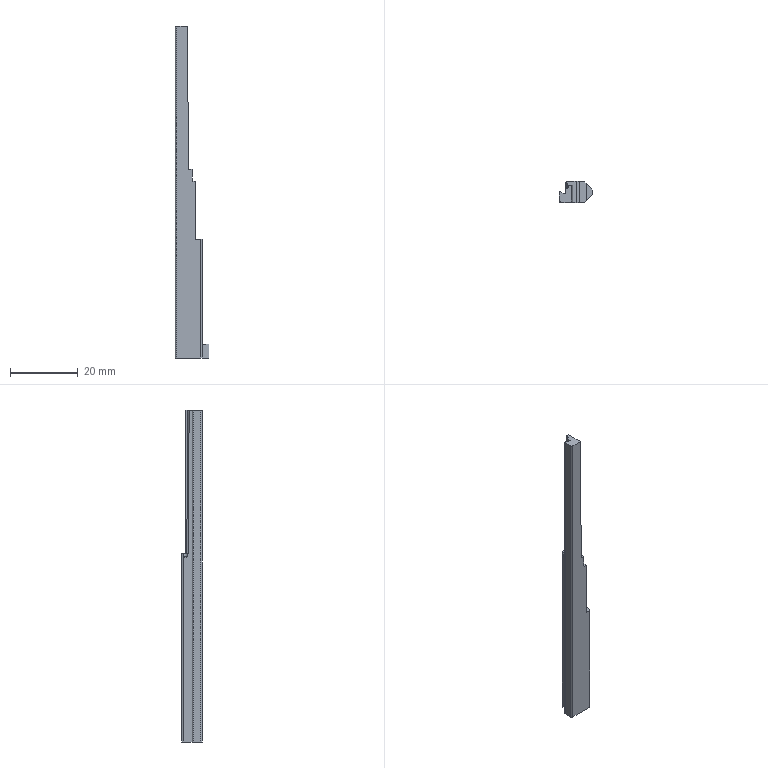Part | Creo | 1 solid | 32 faces | box 10 x 6.2 x 98.191 mm | volume 2714 mm3 | plane 25 | cylinder 5 | cone 2 | commonest cylinder face diameters 0.6 x2 1 x2 1.005 x1
STEP:
#1=CARTESIAN_POINT('',(0.,0.,0.));
#2=DIRECTION('',(0.,0.,1.));
#3=DIRECTION('',(1.,0.,0.));
#4=AXIS2_PLACEMENT_3D('',#1,#2,#3);
#5=CARTESIAN_POINT('',(41.857,15.007,44.101));
#6=VERTEX_POINT('',#5);
#7=CARTESIAN_POINT('',(41.709,15.153,1.79));
#8=VERTEX_POINT('',#7);
#9=CARTESIAN_POINT('',(41.857,15.007,44.101));
#10=DIRECTION('',(-0.003491,0.00346,-1.));
#11=VECTOR('',#10,42.311);
#12=LINE('',#9,#11);
#13=EDGE_CURVE('',#6,#8,#12,.T.);
#14=ORIENTED_EDGE('',*,*,#13,.T.);
#15=CARTESIAN_POINT('',(43.119,15.166,1.79));
#16=VERTEX_POINT('',#15);
#17=CARTESIAN_POINT('',(43.119,15.166,1.79));
#18=DIRECTION('',(-1.,-0.008727,0.));
#19=VECTOR('',#18,1.41);
#20=LINE('',#17,#19);
#21=EDGE_CURVE('',#16,#8,#20,.T.);
#22=ORIENTED_EDGE('',*,*,#21,.F.);
#23=CARTESIAN_POINT('',(42.75,15.015,44.101));
#24=VERTEX_POINT('',#23);
#25=CARTESIAN_POINT('',(42.75,15.015,44.101));
#26=DIRECTION('',(0.008726,0.003567,-1.));
#27=VECTOR('',#26,42.312);
#28=LINE('',#25,#27);
#29=EDGE_CURVE('',#24,#16,#28,.T.);
#30=ORIENTED_EDGE('',*,*,#29,.F.);
#31=CARTESIAN_POINT('',(42.75,15.015,44.101));
#32=DIRECTION('',(-1.,-0.008727,0.));
#33=VECTOR('',#32,0.8934);
#34=LINE('',#31,#33);
#35=EDGE_CURVE('',#24,#6,#34,.T.);
#36=ORIENTED_EDGE('',*,*,#35,.T.);
#37=EDGE_LOOP('',(#14,#22,#30,#36));
#38=FACE_OUTER_BOUND('',#37,.F.);
#39=CARTESIAN_POINT('',(45.746,15.067,36.563));
#40=DIRECTION('',(0.008726,-1.,-0.003491));
#41=DIRECTION('',(1.,0.008727,0.));
#42=AXIS2_PLACEMENT_3D('',#39,#40,#41);
#43=PLANE('',#42);
#44=ADVANCED_FACE('',(#38),#43,.F.);
#45=CARTESIAN_POINT('',(41.709,14.663,1.79));
#46=VERTEX_POINT('',#45);
#47=CARTESIAN_POINT('',(41.857,14.516,44.101));
#48=VERTEX_POINT('',#47);
#49=CARTESIAN_POINT('',(41.709,14.663,1.79));
#50=DIRECTION('',(0.003491,-0.003491,1.));
#51=VECTOR('',#50,42.311);
#52=LINE('',#49,#51);
#53=EDGE_CURVE('',#46,#48,#52,.T.);
#54=ORIENTED_EDGE('',*,*,#53,.F.);
#55=CARTESIAN_POINT('',(41.709,15.153,1.79));
#56=DIRECTION('',(0.,-1.,-0.000000002));
#57=VECTOR('',#56,0.49);
#58=LINE('',#55,#57);
#59=EDGE_CURVE('',#8,#46,#58,.T.);
#60=ORIENTED_EDGE('',*,*,#59,.F.);
#61=ORIENTED_EDGE('',*,*,#13,.F.);
#62=CARTESIAN_POINT('',(41.857,15.007,44.101));
#63=DIRECTION('',(0.,-1.,-0.000000002));
#64=VECTOR('',#63,0.4913);
#65=LINE('',#62,#64);
#66=EDGE_CURVE('',#6,#48,#65,.T.);
#67=ORIENTED_EDGE('',*,*,#66,.T.);
#68=EDGE_LOOP('',(#54,#60,#61,#67));
#69=FACE_OUTER_BOUND('',#68,.F.);
#70=CARTESIAN_POINT('',(41.83,17.654,36.563));
#71=DIRECTION('',(1.,0.,-0.003491));
#72=DIRECTION('',(0.,1.,0.));
#73=AXIS2_PLACEMENT_3D('',#70,#71,#72);
#74=PLANE('',#73);
#75=ADVANCED_FACE('',(#69),#74,.F.);
#76=CARTESIAN_POINT('',(41.354,14.013,44.101));
#77=VERTEX_POINT('',#76);
#78=CARTESIAN_POINT('',(41.206,14.161,1.79));
#79=VERTEX_POINT('',#78);
#80=CARTESIAN_POINT('',(41.354,14.013,44.101));
#81=DIRECTION('',(-0.003491,0.003491,-1.));
#82=VECTOR('',#81,42.311);
#83=LINE('',#80,#82);
#84=EDGE_CURVE('',#77,#79,#83,.T.);
#85=ORIENTED_EDGE('',*,*,#84,.T.);
#86=CARTESIAN_POINT('',(41.709,14.663,1.79));
#87=CARTESIAN_POINT('',(41.709,14.496,1.79));
#88=CARTESIAN_POINT('',(41.582,14.288,1.79));
#89=CARTESIAN_POINT('',(41.374,14.161,1.79));
#90=CARTESIAN_POINT('',(41.206,14.161,1.79));
#91=B_SPLINE_CURVE_WITH_KNOTS('',3,(#86,#87,#88,#89,#90),.UNSPECIFIED.,.F.,.F.,(4,1,4),(0.,0.5,1.),.UNSPECIFIED.);
#92=EDGE_CURVE('',#46,#79,#91,.T.);
#93=ORIENTED_EDGE('',*,*,#92,.F.);
#94=ORIENTED_EDGE('',*,*,#53,.T.);
#95=CARTESIAN_POINT('',(41.354,14.013,44.101));
#96=CARTESIAN_POINT('',(41.522,14.013,44.101));
#97=CARTESIAN_POINT('',(41.73,14.14,44.101));
#98=CARTESIAN_POINT('',(41.857,14.348,44.101));
#99=CARTESIAN_POINT('',(41.857,14.516,44.101));
#100=B_SPLINE_CURVE_WITH_KNOTS('',3,(#95,#96,#97,#98,#99),.UNSPECIFIED.,.F.,.F.,(4,1,4),(0.,0.5,1.),.UNSPECIFIED.);
#101=EDGE_CURVE('',#77,#48,#100,.T.);
#102=ORIENTED_EDGE('',*,*,#101,.F.);
#103=EDGE_LOOP('',(#85,#93,#94,#102));
#104=FACE_OUTER_BOUND('',#103,.F.);
#105=CARTESIAN_POINT('',(40.869,15.001,-94.88));
#106=DIRECTION('',(0.003491,-0.003491,1.));
#107=DIRECTION('',(0.,1.,0.003491));
#108=AXIS2_PLACEMENT_3D('',#105,#106,#107);
#109=CYLINDRICAL_SURFACE('',#108,0.5025);
#110=ADVANCED_FACE('',(#104),#109,.F.);
#111=CARTESIAN_POINT('',(41.127,14.161,1.79));
#112=VERTEX_POINT('',#111);
#113=CARTESIAN_POINT('',(41.206,14.161,1.79));
#114=DIRECTION('',(-1.,0.,0.));
#115=VECTOR('',#114,0.07962);
#116=LINE('',#113,#115);
#117=EDGE_CURVE('',#79,#112,#116,.T.);
#118=ORIENTED_EDGE('',*,*,#117,.F.);
#119=ORIENTED_EDGE('',*,*,#84,.F.);
#120=CARTESIAN_POINT('',(41.127,14.013,44.101));
#121=VERTEX_POINT('',#120);
#122=CARTESIAN_POINT('',(41.354,14.013,44.101));
#123=DIRECTION('',(-1.,0.,0.000000003));
#124=VECTOR('',#123,0.2273);
#125=LINE('',#122,#124);
#126=EDGE_CURVE('',#77,#121,#125,.T.);
#127=ORIENTED_EDGE('',*,*,#126,.T.);
#128=CARTESIAN_POINT('',(41.127,14.013,44.101));
#129=DIRECTION('',(0.,0.003491,-1.));
#130=VECTOR('',#129,42.311);
#131=LINE('',#128,#130);
#132=EDGE_CURVE('',#121,#112,#131,.T.);
#133=ORIENTED_EDGE('',*,*,#132,.T.);
#134=EDGE_LOOP('',(#118,#119,#127,#133));
#135=FACE_OUTER_BOUND('',#134,.F.);
#136=CARTESIAN_POINT('',(44.44,14.039,36.563));
#137=DIRECTION('',(0.,-1.,-0.003491));
#138=DIRECTION('',(1.,0.,0.));
#139=AXIS2_PLACEMENT_3D('',#136,#137,#138);
#140=PLANE('',#139);
#141=ADVANCED_FACE('',(#135),#140,.F.);
#142=CARTESIAN_POINT('',(43.119,10.049,1.79));
#143=VERTEX_POINT('',#142);
#144=CARTESIAN_POINT('',(44.165,10.049,1.79));
#145=VERTEX_POINT('',#144);
#146=CARTESIAN_POINT('',(43.119,10.049,1.79));
#147=DIRECTION('',(1.,0.,0.));
#148=VECTOR('',#147,1.045);
#149=LINE('',#146,#148);
#150=EDGE_CURVE('',#143,#145,#149,.T.);
#151=ORIENTED_EDGE('',*,*,#150,.F.);
#152=CARTESIAN_POINT('',(43.119,10.049,1.79));
#153=DIRECTION('',(0.,1.,0.));
#154=VECTOR('',#153,5.117);
#155=LINE('',#152,#154);
#156=EDGE_CURVE('',#143,#16,#155,.T.);
#157=ORIENTED_EDGE('',*,*,#156,.T.);
#158=ORIENTED_EDGE('',*,*,#21,.T.);
#159=ORIENTED_EDGE('',*,*,#59,.T.);
#160=ORIENTED_EDGE('',*,*,#92,.T.);
#161=ORIENTED_EDGE('',*,*,#117,.T.);
#162=CARTESIAN_POINT('',(41.127,14.552,1.79));
#163=VERTEX_POINT('',#162);
#164=CARTESIAN_POINT('',(41.127,14.161,1.79));
#165=DIRECTION('',(0.,1.,0.));
#166=VECTOR('',#165,0.3912);
#167=LINE('',#164,#166);
#168=EDGE_CURVE('',#112,#163,#167,.T.);
#169=ORIENTED_EDGE('',*,*,#168,.T.);
#170=CARTESIAN_POINT('',(41.127,15.657,1.79));
#171=VERTEX_POINT('',#170);
#172=CARTESIAN_POINT('',(41.127,15.105,1.79));
#173=DIRECTION('',(0.,0.,-1.));
#174=DIRECTION('',(0.,1.,0.));
#175=AXIS2_PLACEMENT_3D('',#172,#173,#174);
#176=CIRCLE('',#175,0.5527);
#177=EDGE_CURVE('',#171,#163,#176,.T.);
#178=ORIENTED_EDGE('',*,*,#177,.F.);
#179=CARTESIAN_POINT('',(41.127,15.749,1.79));
#180=VERTEX_POINT('',#179);
#181=CARTESIAN_POINT('',(41.127,15.657,1.79));
#182=DIRECTION('',(0.,1.,0.));
#183=VECTOR('',#182,0.09123);
#184=LINE('',#181,#183);
#185=EDGE_CURVE('',#171,#180,#184,.T.);
#186=ORIENTED_EDGE('',*,*,#185,.T.);
#187=CARTESIAN_POINT('',(41.627,16.249,1.79));
#188=VERTEX_POINT('',#187);
#189=CARTESIAN_POINT('',(41.627,15.749,1.79));
#190=DIRECTION('',(0.,0.,1.));
#191=DIRECTION('',(0.,1.,0.));
#192=AXIS2_PLACEMENT_3D('',#189,#190,#191);
#193=CIRCLE('',#192,0.5);
#194=EDGE_CURVE('',#188,#180,#193,.T.);
#195=ORIENTED_EDGE('',*,*,#194,.F.);
#196=CARTESIAN_POINT('',(44.165,16.249,1.79));
#197=VERTEX_POINT('',#196);
#198=CARTESIAN_POINT('',(41.627,16.249,1.79));
#199=DIRECTION('',(1.,0.,0.));
#200=VECTOR('',#199,2.538);
#201=LINE('',#198,#200);
#202=EDGE_CURVE('',#188,#197,#201,.T.);
#203=ORIENTED_EDGE('',*,*,#202,.T.);
#204=CARTESIAN_POINT('',(44.165,16.249,1.79));
#205=DIRECTION('',(0.,-1.,0.));
#206=VECTOR('',#205,6.2);
#207=LINE('',#204,#206);
#208=EDGE_CURVE('',#197,#145,#207,.T.);
#209=ORIENTED_EDGE('',*,*,#208,.T.);
#210=EDGE_LOOP('',(#151,#157,#158,#159,#160,#161,#169,#178,#186,#195,#203,#209));
#211=FACE_OUTER_BOUND('',#210,.F.);
#212=CARTESIAN_POINT('',(-0.07825,87.525,1.79));
#213=DIRECTION('',(0.,0.,-1.));
#214=DIRECTION('',(0.,-1.,0.));
#215=AXIS2_PLACEMENT_3D('',#212,#213,#214);
#216=PLANE('',#215);
#217=ADVANCED_FACE('',(#211),#216,.F.);
#218=CARTESIAN_POINT('',(39.627,10.049,-54.09));
#219=VERTEX_POINT('',#218);
#220=CARTESIAN_POINT('',(46.627,10.049,-54.09));
#221=VERTEX_POINT('',#220);
#222=CARTESIAN_POINT('',(39.627,10.049,-54.09));
#223=DIRECTION('',(1.,0.,0.));
#224=VECTOR('',#223,7.);
#225=LINE('',#222,#224);
#226=EDGE_CURVE('',#219,#221,#225,.T.);
#227=ORIENTED_EDGE('',*,*,#226,.F.);
#228=CARTESIAN_POINT('',(39.627,10.049,44.101));
#229=VERTEX_POINT('',#228);
#230=CARTESIAN_POINT('',(39.627,10.049,-54.09));
#231=DIRECTION('',(0.,0.,1.));
#232=VECTOR('',#231,98.191);
#233=LINE('',#230,#232);
#234=EDGE_CURVE('',#219,#229,#233,.T.);
#235=ORIENTED_EDGE('',*,*,#234,.T.);
#236=CARTESIAN_POINT('',(42.75,10.049,44.101));
#237=VERTEX_POINT('',#236);
#238=CARTESIAN_POINT('',(42.75,10.049,44.101));
#239=DIRECTION('',(-1.,0.,0.));
#240=VECTOR('',#239,3.123);
#241=LINE('',#238,#240);
#242=EDGE_CURVE('',#237,#229,#241,.T.);
#243=ORIENTED_EDGE('',*,*,#242,.F.);
#244=CARTESIAN_POINT('',(43.119,10.049,1.79));
#245=DIRECTION('',(-0.008727,0.,1.));
#246=VECTOR('',#245,42.312);
#247=LINE('',#244,#246);
#248=EDGE_CURVE('',#143,#237,#247,.T.);
#249=ORIENTED_EDGE('',*,*,#248,.F.);
#250=ORIENTED_EDGE('',*,*,#150,.T.);
#251=CARTESIAN_POINT('',(44.182,10.049,-0.2173));
#252=VERTEX_POINT('',#251);
#253=CARTESIAN_POINT('',(44.182,10.049,-0.2173));
#254=DIRECTION('',(-0.008727,0.,1.));
#255=VECTOR('',#254,2.008);
#256=LINE('',#253,#255);
#257=EDGE_CURVE('',#252,#145,#256,.T.);
#258=ORIENTED_EDGE('',*,*,#257,.F.);
#259=CARTESIAN_POINT('',(44.295,10.049,-1.827));
#260=VERTEX_POINT('',#259);
#261=CARTESIAN_POINT('',(44.295,10.049,-1.827));
#262=DIRECTION('',(-0.06976,0.,0.9976));
#263=VECTOR('',#262,1.614);
#264=LINE('',#261,#263);
#265=EDGE_CURVE('',#260,#252,#264,.T.);
#266=ORIENTED_EDGE('',*,*,#265,.F.);
#267=CARTESIAN_POINT('',(45.147,10.049,-1.827));
#268=VERTEX_POINT('',#267);
#269=CARTESIAN_POINT('',(45.147,10.049,-1.827));
#270=DIRECTION('',(-1.,0.,0.));
#271=VECTOR('',#270,0.8521);
#272=LINE('',#269,#271);
#273=EDGE_CURVE('',#268,#260,#272,.T.);
#274=ORIENTED_EDGE('',*,*,#273,.F.);
#275=CARTESIAN_POINT('',(45.147,10.049,-19.011));
#276=VERTEX_POINT('',#275);
#277=CARTESIAN_POINT('',(45.147,10.049,-19.011));
#278=DIRECTION('',(0.,0.,1.));
#279=VECTOR('',#278,17.184);
#280=LINE('',#277,#279);
#281=EDGE_CURVE('',#276,#268,#280,.T.);
#282=ORIENTED_EDGE('',*,*,#281,.F.);
#283=CARTESIAN_POINT('',(46.627,10.049,-19.011));
#284=VERTEX_POINT('',#283);
#285=CARTESIAN_POINT('',(45.147,10.049,-19.011));
#286=DIRECTION('',(1.,0.,0.));
#287=VECTOR('',#286,1.48);
#288=LINE('',#285,#287);
#289=EDGE_CURVE('',#276,#284,#288,.T.);
#290=ORIENTED_EDGE('',*,*,#289,.T.);
#291=CARTESIAN_POINT('',(46.627,10.049,-19.011));
#292=DIRECTION('',(0.,0.,-1.));
#293=VECTOR('',#292,35.079);
#294=LINE('',#291,#293);
#295=EDGE_CURVE('',#284,#221,#294,.T.);
#296=ORIENTED_EDGE('',*,*,#295,.T.);
#297=EDGE_LOOP('',(#227,#235,#243,#249,#250,#258,#266,#274,#282,#290,#296));
#298=FACE_OUTER_BOUND('',#297,.F.);
#299=CARTESIAN_POINT('',(40.127,10.049,-45.09));
#300=DIRECTION('',(0.,-1.,0.));
#301=DIRECTION('',(0.,0.,-1.));
#302=AXIS2_PLACEMENT_3D('',#299,#300,#301);
#303=PLANE('',#302);
#304=ADVANCED_FACE('',(#298),#303,.T.);
#305=CARTESIAN_POINT('',(49.127,12.549,-54.09));
#306=VERTEX_POINT('',#305);
#307=CARTESIAN_POINT('',(47.127,10.549,-54.09));
#308=VERTEX_POINT('',#307);
#309=CARTESIAN_POINT('',(49.127,12.549,-54.09));
#310=DIRECTION('',(-0.7071,-0.7071,0.));
#311=VECTOR('',#310,2.828);
#312=LINE('',#309,#311);
#313=EDGE_CURVE('',#306,#308,#312,.T.);
#314=ORIENTED_EDGE('',*,*,#313,.F.);
#315=CARTESIAN_POINT('',(49.127,13.749,-54.09));
#316=VERTEX_POINT('',#315);
#317=CARTESIAN_POINT('',(49.127,13.749,-54.09));
#318=DIRECTION('',(0.,-1.,0.));
#319=VECTOR('',#318,1.2);
#320=LINE('',#317,#319);
#321=EDGE_CURVE('',#316,#306,#320,.T.);
#322=ORIENTED_EDGE('',*,*,#321,.F.);
#323=CARTESIAN_POINT('',(47.127,15.749,-54.09));
#324=VERTEX_POINT('',#323);
#325=CARTESIAN_POINT('',(47.127,15.749,-54.09));
#326=DIRECTION('',(0.7071,-0.7071,0.));
#327=VECTOR('',#326,2.828);
#328=LINE('',#325,#327);
#329=EDGE_CURVE('',#324,#316,#328,.T.);
#330=ORIENTED_EDGE('',*,*,#329,.F.);
#331=CARTESIAN_POINT('',(46.627,16.249,-54.09));
#332=VERTEX_POINT('',#331);
#333=CARTESIAN_POINT('',(46.627,16.249,-54.09));
#334=DIRECTION('',(0.7071,-0.7071,0.));
#335=VECTOR('',#334,0.7071);
#336=LINE('',#333,#335);
#337=EDGE_CURVE('',#332,#324,#336,.T.);
#338=ORIENTED_EDGE('',*,*,#337,.F.);
#339=CARTESIAN_POINT('',(41.627,16.249,-54.09));
#340=VERTEX_POINT('',#339);
#341=CARTESIAN_POINT('',(41.627,16.249,-54.09));
#342=DIRECTION('',(1.,0.,0.));
#343=VECTOR('',#342,5.);
#344=LINE('',#341,#343);
#345=EDGE_CURVE('',#340,#332,#344,.T.);
#346=ORIENTED_EDGE('',*,*,#345,.F.);
#347=CARTESIAN_POINT('',(41.127,15.749,-54.09));
#348=VERTEX_POINT('',#347);
#349=CARTESIAN_POINT('',(41.627,15.749,-54.09));
#350=DIRECTION('',(0.,0.,-1.));
#351=DIRECTION('',(-1.,0.,0.));
#352=AXIS2_PLACEMENT_3D('',#349,#350,#351);
#353=CIRCLE('',#352,0.5);
#354=EDGE_CURVE('',#348,#340,#353,.T.);
#355=ORIENTED_EDGE('',*,*,#354,.F.);
#356=CARTESIAN_POINT('',(41.127,12.823,-54.09));
#357=VERTEX_POINT('',#356);
#358=CARTESIAN_POINT('',(41.127,12.823,-54.09));
#359=DIRECTION('',(0.,1.,0.));
#360=VECTOR('',#359,2.926);
#361=LINE('',#358,#360);
#362=EDGE_CURVE('',#357,#348,#361,.T.);
#363=ORIENTED_EDGE('',*,*,#362,.F.);
#364=CARTESIAN_POINT('',(40.7,12.551,-54.09));
#365=VERTEX_POINT('',#364);
#366=CARTESIAN_POINT('',(40.827,12.823,-54.09));
#367=DIRECTION('',(0.,0.,1.));
#368=DIRECTION('',(-0.4226,-0.9063,0.));
#369=AXIS2_PLACEMENT_3D('',#366,#367,#368);
#370=CIRCLE('',#369,0.3);
#371=EDGE_CURVE('',#365,#357,#370,.T.);
#372=ORIENTED_EDGE('',*,*,#371,.F.);
#373=CARTESIAN_POINT('',(39.554,13.086,-54.09));
#374=VERTEX_POINT('',#373);
#375=CARTESIAN_POINT('',(39.554,13.086,-54.09));
#376=DIRECTION('',(0.9063,-0.4226,0.));
#377=VECTOR('',#376,1.265);
#378=LINE('',#375,#377);
#379=EDGE_CURVE('',#374,#365,#378,.T.);
#380=ORIENTED_EDGE('',*,*,#379,.F.);
#381=CARTESIAN_POINT('',(39.127,12.814,-54.09));
#382=VERTEX_POINT('',#381);
#383=CARTESIAN_POINT('',(39.427,12.814,-54.09));
#384=DIRECTION('',(0.,0.,-1.));
#385=DIRECTION('',(-1.,0.,0.));
#386=AXIS2_PLACEMENT_3D('',#383,#384,#385);
#387=CIRCLE('',#386,0.3);
#388=EDGE_CURVE('',#382,#374,#387,.T.);
#389=ORIENTED_EDGE('',*,*,#388,.F.);
#390=CARTESIAN_POINT('',(39.127,10.549,-54.09));
#391=VERTEX_POINT('',#390);
#392=CARTESIAN_POINT('',(39.127,12.814,-54.09));
#393=DIRECTION('',(0.,-1.,0.));
#394=VECTOR('',#393,2.265);
#395=LINE('',#392,#394);
#396=EDGE_CURVE('',#382,#391,#395,.T.);
#397=ORIENTED_EDGE('',*,*,#396,.T.);
#398=CARTESIAN_POINT('',(39.627,10.549,-54.09));
#399=DIRECTION('',(0.,0.,-1.));
#400=DIRECTION('',(0.,-1.,0.));
#401=AXIS2_PLACEMENT_3D('',#398,#399,#400);
#402=CIRCLE('',#401,0.5);
#403=EDGE_CURVE('',#219,#391,#402,.T.);
#404=ORIENTED_EDGE('',*,*,#403,.F.);
#405=ORIENTED_EDGE('',*,*,#226,.T.);
#406=CARTESIAN_POINT('',(47.127,10.549,-54.09));
#407=DIRECTION('',(-0.7071,-0.7071,0.));
#408=VECTOR('',#407,0.7071);
#409=LINE('',#406,#408);
#410=EDGE_CURVE('',#308,#221,#409,.T.);
#411=ORIENTED_EDGE('',*,*,#410,.F.);
#412=EDGE_LOOP('',(#314,#322,#330,#338,#346,#355,#363,#372,#380,#389,#397,#404,#405,#411));
#413=FACE_OUTER_BOUND('',#412,.F.);
#414=CARTESIAN_POINT('',(0.,0.,-54.09));
#415=DIRECTION('',(0.,0.,-1.));
#416=DIRECTION('',(-1.,0.,0.));
#417=AXIS2_PLACEMENT_3D('',#414,#415,#416);
#418=PLANE('',#417);
#419=ADVANCED_FACE('',(#413),#418,.T.);
#420=ORIENTED_EDGE('',*,*,#313,.T.);
#421=CARTESIAN_POINT('',(47.127,10.549,-50.09));
#422=VERTEX_POINT('',#421);
#423=CARTESIAN_POINT('',(47.127,10.549,-54.09));
#424=DIRECTION('',(0.,0.,1.));
#425=VECTOR('',#424,4.);
#426=LINE('',#423,#425);
#427=EDGE_CURVE('',#308,#422,#426,.T.);
#428=ORIENTED_EDGE('',*,*,#427,.T.);
#429=CARTESIAN_POINT('',(49.127,12.549,-50.09));
#430=VERTEX_POINT('',#429);
#431=CARTESIAN_POINT('',(47.127,10.549,-50.09));
#432=DIRECTION('',(0.7071,0.7071,0.));
#433=VECTOR('',#432,2.828);
#434=LINE('',#431,#433);
#435=EDGE_CURVE('',#422,#430,#434,.T.);
#436=ORIENTED_EDGE('',*,*,#435,.T.);
#437=CARTESIAN_POINT('',(49.127,12.549,-54.09));
#438=DIRECTION('',(0.,0.,1.));
#439=VECTOR('',#438,4.);
#440=LINE('',#437,#439);
#441=EDGE_CURVE('',#306,#430,#440,.T.);
#442=ORIENTED_EDGE('',*,*,#441,.F.);
#443=EDGE_LOOP('',(#420,#428,#436,#442));
#444=FACE_OUTER_BOUND('',#443,.F.);
#445=CARTESIAN_POINT('',(47.127,10.549,-54.09));
#446=DIRECTION('',(-0.7071,0.7071,0.));
#447=DIRECTION('',(0.,0.,1.));
#448=AXIS2_PLACEMENT_3D('',#445,#446,#447);
#449=PLANE('',#448);
#450=ADVANCED_FACE('',(#444),#449,.F.);
#451=ORIENTED_EDGE('',*,*,#427,.F.);
#452=ORIENTED_EDGE('',*,*,#410,.T.);
#453=ORIENTED_EDGE('',*,*,#295,.F.);
#454=CARTESIAN_POINT('',(47.127,10.549,-19.011));
#455=VERTEX_POINT('',#454);
#456=CARTESIAN_POINT('',(46.627,10.049,-19.011));
#457=DIRECTION('',(0.7071,0.7071,0.));
#458=VECTOR('',#457,0.7071);
#459=LINE('',#456,#458);
#460=EDGE_CURVE('',#284,#455,#459,.T.);
#461=ORIENTED_EDGE('',*,*,#460,.T.);
#462=CARTESIAN_POINT('',(47.127,10.549,-50.09));
#463=DIRECTION('',(0.,0.,1.));
#464=VECTOR('',#463,31.079);
#465=LINE('',#462,#464);
#466=EDGE_CURVE('',#422,#455,#465,.T.);
#467=ORIENTED_EDGE('',*,*,#466,.F.);
#468=EDGE_LOOP('',(#451,#452,#453,#461,#467));
#469=FACE_OUTER_BOUND('',#468,.F.);
#470=CARTESIAN_POINT('',(46.627,10.049,-45.09));
#471=DIRECTION('',(0.7071,-0.7071,0.));
#472=DIRECTION('',(0.,0.,-1.));
#473=AXIS2_PLACEMENT_3D('',#470,#471,#472);
#474=PLANE('',#473);
#475=ADVANCED_FACE('',(#469),#474,.T.);
#476=ORIENTED_EDGE('',*,*,#289,.F.);
#477=CARTESIAN_POINT('',(45.147,16.249,-19.011));
#478=VERTEX_POINT('',#477);
#479=CARTESIAN_POINT('',(45.147,10.049,-19.011));
#480=DIRECTION('',(0.,1.,0.));
#481=VECTOR('',#480,6.2);
#482=LINE('',#479,#481);
#483=EDGE_CURVE('',#276,#478,#482,.T.);
#484=ORIENTED_EDGE('',*,*,#483,.T.);
#485=CARTESIAN_POINT('',(46.627,16.249,-19.011));
#486=VERTEX_POINT('',#485);
#487=CARTESIAN_POINT('',(45.147,16.249,-19.011));
#488=DIRECTION('',(1.,0.,0.));
#489=VECTOR('',#488,1.48);
#490=LINE('',#487,#489);
#491=EDGE_CURVE('',#478,#486,#490,.T.);
#492=ORIENTED_EDGE('',*,*,#491,.T.);
#493=CARTESIAN_POINT('',(47.127,15.749,-19.011));
#494=VERTEX_POINT('',#493);
#495=CARTESIAN_POINT('',(47.127,15.749,-19.011));
#496=DIRECTION('',(-0.7071,0.7071,0.));
#497=VECTOR('',#496,0.7071);
#498=LINE('',#495,#497);
#499=EDGE_CURVE('',#494,#486,#498,.T.);
#500=ORIENTED_EDGE('',*,*,#499,.F.);
#501=CARTESIAN_POINT('',(47.127,15.749,-19.011));
#502=DIRECTION('',(0.,-1.,0.));
#503=VECTOR('',#502,5.2);
#504=LINE('',#501,#503);
#505=EDGE_CURVE('',#494,#455,#504,.T.);
#506=ORIENTED_EDGE('',*,*,#505,.T.);
#507=ORIENTED_EDGE('',*,*,#460,.F.);
#508=EDGE_LOOP('',(#476,#484,#492,#500,#506,#507));
#509=FACE_OUTER_BOUND('',#508,.F.);
#510=CARTESIAN_POINT('',(44.092,76.118,-19.011));
#511=DIRECTION('',(0.,0.,-1.));
#512=DIRECTION('',(0.,-1.,0.));
#513=AXIS2_PLACEMENT_3D('',#510,#511,#512);
#514=PLANE('',#513);
#515=ADVANCED_FACE('',(#509),#514,.F.);
#516=CARTESIAN_POINT('',(45.147,16.249,-1.827));
#517=VERTEX_POINT('',#516);
#518=CARTESIAN_POINT('',(45.147,16.249,-1.827));
#519=DIRECTION('',(0.,-1.,0.));
#520=VECTOR('',#519,6.2);
#521=LINE('',#518,#520);
#522=EDGE_CURVE('',#517,#268,#521,.T.);
#523=ORIENTED_EDGE('',*,*,#522,.F.);
#524=CARTESIAN_POINT('',(45.147,16.249,-19.011));
#525=DIRECTION('',(0.,0.,1.));
#526=VECTOR('',#525,17.184);
#527=LINE('',#524,#526);
#528=EDGE_CURVE('',#478,#517,#527,.T.);
#529=ORIENTED_EDGE('',*,*,#528,.F.);
#530=ORIENTED_EDGE('',*,*,#483,.F.);
#531=ORIENTED_EDGE('',*,*,#281,.T.);
#532=EDGE_LOOP('',(#523,#529,#530,#531));
#533=FACE_OUTER_BOUND('',#532,.F.);
#534=CARTESIAN_POINT('',(45.147,85.314,-1.827));
#535=DIRECTION('',(1.,0.,0.));
#536=DIRECTION('',(0.,1.,0.));
#537=AXIS2_PLACEMENT_3D('',#534,#535,#536);
#538=PLANE('',#537);
#539=ADVANCED_FACE('',(#533),#538,.T.);
#540=CARTESIAN_POINT('',(44.295,16.249,-1.827));
#541=VERTEX_POINT('',#540);
#542=CARTESIAN_POINT('',(44.295,16.249,-1.827));
#543=DIRECTION('',(0.,-1.,0.));
#544=VECTOR('',#543,6.2);
#545=LINE('',#542,#544);
#546=EDGE_CURVE('',#541,#260,#545,.T.);
#547=ORIENTED_EDGE('',*,*,#546,.F.);
#548=CARTESIAN_POINT('',(45.147,16.249,-1.827));
#549=DIRECTION('',(-1.,0.,0.));
#550=VECTOR('',#549,0.8521);
#551=LINE('',#548,#550);
#552=EDGE_CURVE('',#517,#541,#551,.T.);
#553=ORIENTED_EDGE('',*,*,#552,.F.);
#554=ORIENTED_EDGE('',*,*,#522,.T.);
#555=ORIENTED_EDGE('',*,*,#273,.T.);
#556=EDGE_LOOP('',(#547,#553,#554,#555));
#557=FACE_OUTER_BOUND('',#556,.F.);
#558=CARTESIAN_POINT('',(-45.303,87.525,-1.827));
#559=DIRECTION('',(0.,0.,1.));
#560=DIRECTION('',(-1.,0.,0.));
#561=AXIS2_PLACEMENT_3D('',#558,#559,#560);
#562=PLANE('',#561);
#563=ADVANCED_FACE('',(#557),#562,.T.);
#564=CARTESIAN_POINT('',(44.182,16.249,-0.2173));
#565=VERTEX_POINT('',#564);
#566=CARTESIAN_POINT('',(44.182,16.249,-0.2173));
#567=DIRECTION('',(0.,-1.,0.));
#568=VECTOR('',#567,6.2);
#569=LINE('',#566,#568);
#570=EDGE_CURVE('',#565,#252,#569,.T.);
#571=ORIENTED_EDGE('',*,*,#570,.F.);
#572=CARTESIAN_POINT('',(44.182,16.249,-0.2173));
#573=DIRECTION('',(0.06976,0.,-0.9976));
#574=VECTOR('',#573,1.614);
#575=LINE('',#572,#574);
#576=EDGE_CURVE('',#565,#541,#575,.T.);
#577=ORIENTED_EDGE('',*,*,#576,.T.);
#578=ORIENTED_EDGE('',*,*,#546,.T.);
#579=ORIENTED_EDGE('',*,*,#265,.T.);
#580=EDGE_LOOP('',(#571,#577,#578,#579));
#581=FACE_OUTER_BOUND('',#580,.F.);
#582=CARTESIAN_POINT('',(44.182,86.621,-0.2155));
#583=DIRECTION('',(0.9976,0.,0.06976));
#584=DIRECTION('',(0.,-1.,0.));
#585=AXIS2_PLACEMENT_3D('',#582,#583,#584);
#586=PLANE('',#585);
#587=ADVANCED_FACE('',(#581),#586,.T.);
#588=ORIENTED_EDGE('',*,*,#208,.F.);
#589=CARTESIAN_POINT('',(44.182,16.249,-0.2173));
#590=DIRECTION('',(-0.008727,0.,1.));
#591=VECTOR('',#590,2.008);
#592=LINE('',#589,#591);
#593=EDGE_CURVE('',#565,#197,#592,.T.);
#594=ORIENTED_EDGE('',*,*,#593,.F.);
#595=ORIENTED_EDGE('',*,*,#570,.T.);
#596=ORIENTED_EDGE('',*,*,#257,.T.);
#597=EDGE_LOOP('',(#588,#594,#595,#596));
#598=FACE_OUTER_BOUND('',#597,.F.);
#599=CARTESIAN_POINT('',(44.182,86.621,-0.2191));
#600=DIRECTION('',(1.,0.,0.008727));
#601=DIRECTION('',(0.,-1.,0.));
#602=AXIS2_PLACEMENT_3D('',#599,#600,#601);
#603=PLANE('',#602);
#604=ADVANCED_FACE('',(#598),#603,.T.);
#605=ORIENTED_EDGE('',*,*,#491,.F.);
#606=ORIENTED_EDGE('',*,*,#528,.T.);
#607=ORIENTED_EDGE('',*,*,#552,.T.);
#608=ORIENTED_EDGE('',*,*,#576,.F.);
#609=ORIENTED_EDGE('',*,*,#593,.T.);
#610=ORIENTED_EDGE('',*,*,#202,.F.);
#611=CARTESIAN_POINT('',(41.627,16.249,1.79));
#612=DIRECTION('',(0.,0.,-1.));
#613=VECTOR('',#612,55.88);
#614=LINE('',#611,#613);
#615=EDGE_CURVE('',#188,#340,#614,.T.);
#616=ORIENTED_EDGE('',*,*,#615,.T.);
#617=ORIENTED_EDGE('',*,*,#345,.T.);
#618=CARTESIAN_POINT('',(46.627,16.249,-54.09));
#619=DIRECTION('',(0.,0.,1.));
#620=VECTOR('',#619,35.079);
#621=LINE('',#618,#620);
#622=EDGE_CURVE('',#332,#486,#621,.T.);
#623=ORIENTED_EDGE('',*,*,#622,.T.);
#624=EDGE_LOOP('',(#605,#606,#607,#608,#609,#610,#616,#617,#623));
#625=FACE_OUTER_BOUND('',#624,.F.);
#626=CARTESIAN_POINT('',(47.127,16.249,58.91));
#627=DIRECTION('',(0.,-1.,0.));
#628=DIRECTION('',(0.,0.,-1.));
#629=AXIS2_PLACEMENT_3D('',#626,#627,#628);
#630=PLANE('',#629);
#631=ADVANCED_FACE('',(#625),#630,.F.);
#632=CARTESIAN_POINT('',(41.127,15.749,-54.09));
#633=DIRECTION('',(0.,0.,1.));
#634=VECTOR('',#633,55.88);
#635=LINE('',#632,#634);
#636=EDGE_CURVE('',#348,#180,#635,.T.);
#637=ORIENTED_EDGE('',*,*,#636,.F.);
#638=ORIENTED_EDGE('',*,*,#354,.T.);
#639=ORIENTED_EDGE('',*,*,#615,.F.);
#640=ORIENTED_EDGE('',*,*,#194,.T.);
#641=EDGE_LOOP('',(#637,#638,#639,#640));
#642=FACE_OUTER_BOUND('',#641,.F.);
#643=CARTESIAN_POINT('',(41.627,15.749,58.91));
#644=DIRECTION('',(0.,0.,-1.));
#645=DIRECTION('',(-1.,0.,0.));
#646=AXIS2_PLACEMENT_3D('',#643,#644,#645);
#647=CYLINDRICAL_SURFACE('',#646,0.5);
#648=ADVANCED_FACE('',(#642),#647,.T.);
#649=CARTESIAN_POINT('',(41.127,12.823,44.101));
#650=VERTEX_POINT('',#649);
#651=CARTESIAN_POINT('',(41.127,12.823,44.101));
#652=DIRECTION('',(0.,0.,-1.));
#653=VECTOR('',#652,98.191);
#654=LINE('',#651,#653);
#655=EDGE_CURVE('',#650,#357,#654,.T.);
#656=ORIENTED_EDGE('',*,*,#655,.T.);
#657=ORIENTED_EDGE('',*,*,#362,.T.);
#658=ORIENTED_EDGE('',*,*,#636,.T.);
#659=ORIENTED_EDGE('',*,*,#185,.F.);
#660=CARTESIAN_POINT('',(41.127,15.649,0.7855));
#661=VERTEX_POINT('',#660);
#662=CARTESIAN_POINT('',(41.127,15.649,0.7855));
#663=DIRECTION('',(0.,0.008727,1.));
#664=VECTOR('',#663,1.005);
#665=LINE('',#662,#664);
#666=EDGE_CURVE('',#661,#171,#665,.T.);
#667=ORIENTED_EDGE('',*,*,#666,.F.);
#668=CARTESIAN_POINT('',(41.127,15.345,0.484));
#669=VERTEX_POINT('',#668);
#670=CARTESIAN_POINT('',(41.127,15.345,0.484));
#671=DIRECTION('',(0.,0.7102,0.704));
#672=VECTOR('',#671,0.4282);
#673=LINE('',#670,#672);
#674=EDGE_CURVE('',#669,#661,#673,.T.);
#675=ORIENTED_EDGE('',*,*,#674,.F.);
#676=CARTESIAN_POINT('',(41.127,14.865,0.484));
#677=VERTEX_POINT('',#676);
#678=CARTESIAN_POINT('',(41.127,14.865,0.484));
#679=DIRECTION('',(0.,1.,0.));
#680=VECTOR('',#679,0.4797);
#681=LINE('',#678,#680);
#682=EDGE_CURVE('',#677,#669,#681,.T.);
#683=ORIENTED_EDGE('',*,*,#682,.F.);
#684=CARTESIAN_POINT('',(41.127,14.561,0.7855));
#685=VERTEX_POINT('',#684);
#686=CARTESIAN_POINT('',(41.127,14.561,0.7855));
#687=DIRECTION('',(0.,0.7102,-0.704));
#688=VECTOR('',#687,0.4282);
#689=LINE('',#686,#688);
#690=EDGE_CURVE('',#685,#677,#689,.T.);
#691=ORIENTED_EDGE('',*,*,#690,.F.);
#692=CARTESIAN_POINT('',(41.127,14.552,1.79));
#693=DIRECTION('',(0.,0.008727,-1.));
#694=VECTOR('',#693,1.005);
#695=LINE('',#692,#694);
#696=EDGE_CURVE('',#163,#685,#695,.T.);
#697=ORIENTED_EDGE('',*,*,#696,.F.);
#698=ORIENTED_EDGE('',*,*,#168,.F.);
#699=ORIENTED_EDGE('',*,*,#132,.F.);
#700=CARTESIAN_POINT('',(41.127,14.013,44.101));
#701=DIRECTION('',(0.,-1.,0.));
#702=VECTOR('',#701,1.19);
#703=LINE('',#700,#702);
#704=EDGE_CURVE('',#121,#650,#703,.T.);
#705=ORIENTED_EDGE('',*,*,#704,.T.);
#706=EDGE_LOOP('',(#656,#657,#658,#659,#667,#675,#683,#691,#697,#698,#699,#705));
#707=FACE_OUTER_BOUND('',#706,.F.);
#708=CARTESIAN_POINT('',(41.127,16.249,58.91));
#709=DIRECTION('',(1.,0.,0.));
#710=DIRECTION('',(0.,0.,-1.));
#711=AXIS2_PLACEMENT_3D('',#708,#709,#710);
#712=PLANE('',#711);
#713=ADVANCED_FACE('',(#707),#712,.F.);
#714=CARTESIAN_POINT('',(40.7,12.551,44.101));
#715=VERTEX_POINT('',#714);
#716=CARTESIAN_POINT('',(40.7,12.551,-54.09));
#717=DIRECTION('',(0.,0.,1.));
#718=VECTOR('',#717,98.191);
#719=LINE('',#716,#718);
#720=EDGE_CURVE('',#365,#715,#719,.T.);
#721=ORIENTED_EDGE('',*,*,#720,.F.);
#722=ORIENTED_EDGE('',*,*,#371,.T.);
#723=ORIENTED_EDGE('',*,*,#655,.F.);
#724=CARTESIAN_POINT('',(40.827,12.823,44.101));
#725=DIRECTION('',(0.,0.,-1.));
#726=DIRECTION('',(1.,0.,0.));
#727=AXIS2_PLACEMENT_3D('',#724,#725,#726);
#728=CIRCLE('',#727,0.3);
#729=EDGE_CURVE('',#650,#715,#728,.T.);
#730=ORIENTED_EDGE('',*,*,#729,.T.);
#731=EDGE_LOOP('',(#721,#722,#723,#730));
#732=FACE_OUTER_BOUND('',#731,.F.);
#733=CARTESIAN_POINT('',(40.827,12.823,58.91));
#734=DIRECTION('',(0.,0.,-1.));
#735=DIRECTION('',(-1.,0.,0.));
#736=AXIS2_PLACEMENT_3D('',#733,#734,#735);
#737=CYLINDRICAL_SURFACE('',#736,0.3);
#738=ADVANCED_FACE('',(#732),#737,.F.);
#739=CARTESIAN_POINT('',(39.554,13.086,44.101));
#740=VERTEX_POINT('',#739);
#741=CARTESIAN_POINT('',(40.7,12.551,44.101));
#742=DIRECTION('',(-0.9063,0.4226,0.));
#743=VECTOR('',#742,1.265);
#744=LINE('',#741,#743);
#745=EDGE_CURVE('',#715,#740,#744,.T.);
#746=ORIENTED_EDGE('',*,*,#745,.T.);
#747=CARTESIAN_POINT('',(39.554,13.086,44.101));
#748=DIRECTION('',(0.,0.,-1.));
#749=VECTOR('',#748,98.191);
#750=LINE('',#747,#749);
#751=EDGE_CURVE('',#740,#374,#750,.T.);
#752=ORIENTED_EDGE('',*,*,#751,.T.);
#753=ORIENTED_EDGE('',*,*,#379,.T.);
#754=ORIENTED_EDGE('',*,*,#720,.T.);
#755=EDGE_LOOP('',(#746,#752,#753,#754));
#756=FACE_OUTER_BOUND('',#755,.F.);
#757=CARTESIAN_POINT('',(39.127,13.285,-45.09));
#758=DIRECTION('',(-0.4226,-0.9063,0.));
#759=DIRECTION('',(0.9063,-0.4226,0.));
#760=AXIS2_PLACEMENT_3D('',#757,#758,#759);
#761=PLANE('',#760);
#762=ADVANCED_FACE('',(#756),#761,.F.);
#763=ORIENTED_EDGE('',*,*,#704,.F.);
#764=ORIENTED_EDGE('',*,*,#126,.F.);
#765=ORIENTED_EDGE('',*,*,#101,.T.);
#766=ORIENTED_EDGE('',*,*,#66,.F.);
#767=ORIENTED_EDGE('',*,*,#35,.F.);
#768=CARTESIAN_POINT('',(42.75,10.049,44.101));
#769=DIRECTION('',(0.,1.,0.));
#770=VECTOR('',#769,4.966);
#771=LINE('',#768,#770);
#772=EDGE_CURVE('',#237,#24,#771,.T.);
#773=ORIENTED_EDGE('',*,*,#772,.F.);
#774=ORIENTED_EDGE('',*,*,#242,.T.);
#775=CARTESIAN_POINT('',(39.127,10.549,44.101));
#776=VERTEX_POINT('',#775);
#777=CARTESIAN_POINT('',(39.627,10.549,44.101));
#778=DIRECTION('',(0.,0.,1.));
#779=DIRECTION('',(-1.,0.,0.));
#780=AXIS2_PLACEMENT_3D('',#777,#778,#779);
#781=CIRCLE('',#780,0.5);
#782=EDGE_CURVE('',#776,#229,#781,.T.);
#783=ORIENTED_EDGE('',*,*,#782,.F.);
#784=CARTESIAN_POINT('',(39.127,12.814,44.101));
#785=VERTEX_POINT('',#784);
#786=CARTESIAN_POINT('',(39.127,10.549,44.101));
#787=DIRECTION('',(0.,1.,0.));
#788=VECTOR('',#787,2.265);
#789=LINE('',#786,#788);
#790=EDGE_CURVE('',#776,#785,#789,.T.);
#791=ORIENTED_EDGE('',*,*,#790,.T.);
#792=CARTESIAN_POINT('',(39.427,12.814,44.101));
#793=DIRECTION('',(0.,0.,1.));
#794=DIRECTION('',(0.4226,0.9063,0.));
#795=AXIS2_PLACEMENT_3D('',#792,#793,#794);
#796=CIRCLE('',#795,0.3);
#797=EDGE_CURVE('',#740,#785,#796,.T.);
#798=ORIENTED_EDGE('',*,*,#797,.F.);
#799=ORIENTED_EDGE('',*,*,#745,.F.);
#800=ORIENTED_EDGE('',*,*,#729,.F.);
#801=EDGE_LOOP('',(#763,#764,#765,#766,#767,#773,#774,#783,#791,#798,#799,#800));
#802=FACE_OUTER_BOUND('',#801,.F.);
#803=CARTESIAN_POINT('',(17.66,-88.35,44.101));
#804=DIRECTION('',(0.,0.,1.));
#805=DIRECTION('',(-1.,0.,0.));
#806=AXIS2_PLACEMENT_3D('',#803,#804,#805);
#807=PLANE('',#806);
#808=ADVANCED_FACE('',(#802),#807,.T.);
#809=ORIENTED_EDGE('',*,*,#772,.T.);
#810=ORIENTED_EDGE('',*,*,#29,.T.);
#811=ORIENTED_EDGE('',*,*,#156,.F.);
#812=ORIENTED_EDGE('',*,*,#248,.T.);
#813=EDGE_LOOP('',(#809,#810,#811,#812));
#814=FACE_OUTER_BOUND('',#813,.F.);
#815=CARTESIAN_POINT('',(43.137,-90.96,-0.2195));
#816=DIRECTION('',(1.,0.,0.008727));
#817=DIRECTION('',(0.,1.,0.));
#818=AXIS2_PLACEMENT_3D('',#815,#816,#817);
#819=PLANE('',#818);
#820=ADVANCED_FACE('',(#814),#819,.T.);
#821=ORIENTED_EDGE('',*,*,#782,.T.);
#822=ORIENTED_EDGE('',*,*,#234,.F.);
#823=ORIENTED_EDGE('',*,*,#403,.T.);
#824=CARTESIAN_POINT('',(39.127,10.549,44.101));
#825=DIRECTION('',(0.,0.,-1.));
#826=VECTOR('',#825,98.191);
#827=LINE('',#824,#826);
#828=EDGE_CURVE('',#776,#391,#827,.T.);
#829=ORIENTED_EDGE('',*,*,#828,.F.);
#830=EDGE_LOOP('',(#821,#822,#823,#829));
#831=FACE_OUTER_BOUND('',#830,.F.);
#832=CARTESIAN_POINT('',(39.627,10.549,-45.09));
#833=DIRECTION('',(0.,0.,1.));
#834=DIRECTION('',(1.,0.,0.));
#835=AXIS2_PLACEMENT_3D('',#832,#833,#834);
#836=CYLINDRICAL_SURFACE('',#835,0.5);
#837=ADVANCED_FACE('',(#831),#836,.T.);
#838=ORIENTED_EDGE('',*,*,#790,.F.);
#839=ORIENTED_EDGE('',*,*,#828,.T.);
#840=ORIENTED_EDGE('',*,*,#396,.F.);
#841=CARTESIAN_POINT('',(39.127,12.814,-54.09));
#842=DIRECTION('',(0.,0.,1.));
#843=VECTOR('',#842,98.191);
#844=LINE('',#841,#843);
#845=EDGE_CURVE('',#382,#785,#844,.T.);
#846=ORIENTED_EDGE('',*,*,#845,.T.);
#847=EDGE_LOOP('',(#838,#839,#840,#846));
#848=FACE_OUTER_BOUND('',#847,.F.);
#849=CARTESIAN_POINT('',(39.127,11.499,-45.09));
#850=DIRECTION('',(-1.,0.,0.));
#851=DIRECTION('',(0.,0.,1.));
#852=AXIS2_PLACEMENT_3D('',#849,#850,#851);
#853=PLANE('',#852);
#854=ADVANCED_FACE('',(#848),#853,.T.);
#855=ORIENTED_EDGE('',*,*,#797,.T.);
#856=ORIENTED_EDGE('',*,*,#845,.F.);
#857=ORIENTED_EDGE('',*,*,#388,.T.);
#858=ORIENTED_EDGE('',*,*,#751,.F.);
#859=EDGE_LOOP('',(#855,#856,#857,#858));
#860=FACE_OUTER_BOUND('',#859,.F.);
#861=CARTESIAN_POINT('',(39.427,12.814,-45.09));
#862=DIRECTION('',(0.,0.,-1.));
#863=DIRECTION('',(-1.,0.,0.));
#864=AXIS2_PLACEMENT_3D('',#861,#862,#863);
#865=CYLINDRICAL_SURFACE('',#864,0.3);
#866=ADVANCED_FACE('',(#860),#865,.T.);
#867=ORIENTED_EDGE('',*,*,#177,.T.);
#868=ORIENTED_EDGE('',*,*,#696,.T.);
#869=CARTESIAN_POINT('',(41.671,15.105,0.7855));
#870=VERTEX_POINT('',#869);
#871=CARTESIAN_POINT('',(41.127,15.105,0.7855));
#872=DIRECTION('',(0.,0.,-1.));
#873=DIRECTION('',(1.,0.,0.));
#874=AXIS2_PLACEMENT_3D('',#871,#872,#873);
#875=CIRCLE('',#874,0.544);
#876=EDGE_CURVE('',#870,#685,#875,.T.);
#877=ORIENTED_EDGE('',*,*,#876,.F.);
#878=CARTESIAN_POINT('',(41.127,15.105,0.7855));
#879=DIRECTION('',(0.,0.,-1.));
#880=DIRECTION('',(0.,1.,0.));
#881=AXIS2_PLACEMENT_3D('',#878,#879,#880);
#882=CIRCLE('',#881,0.544);
#883=EDGE_CURVE('',#661,#870,#882,.T.);
#884=ORIENTED_EDGE('',*,*,#883,.F.);
#885=ORIENTED_EDGE('',*,*,#666,.T.);
#886=EDGE_LOOP('',(#867,#868,#877,#884,#885));
#887=FACE_OUTER_BOUND('',#886,.F.);
#888=CARTESIAN_POINT('',(41.127,15.105,1.288));
#889=DIRECTION('',(0.,0.,1.));
#890=DIRECTION('',(0.,1.,0.));
#891=AXIS2_PLACEMENT_3D('',#888,#889,#890);
#892=CONICAL_SURFACE('',#891,0.5484,0.5);
#893=ADVANCED_FACE('',(#887),#892,.F.);
#894=ORIENTED_EDGE('',*,*,#876,.T.);
#895=ORIENTED_EDGE('',*,*,#690,.T.);
#896=CARTESIAN_POINT('',(41.127,15.105,0.484));
#897=DIRECTION('',(0.,0.,1.));
#898=DIRECTION('',(0.,-1.,0.));
#899=AXIS2_PLACEMENT_3D('',#896,#897,#898);
#900=CIRCLE('',#899,0.2398);
#901=EDGE_CURVE('',#677,#669,#900,.T.);
#902=ORIENTED_EDGE('',*,*,#901,.T.);
#903=ORIENTED_EDGE('',*,*,#674,.T.);
#904=ORIENTED_EDGE('',*,*,#883,.T.);
#905=EDGE_LOOP('',(#894,#895,#902,#903,#904));
#906=FACE_OUTER_BOUND('',#905,.F.);
#907=CARTESIAN_POINT('',(41.127,15.105,0.6347));
#908=DIRECTION('',(0.,0.,1.));
#909=DIRECTION('',(-1.,0.,0.));
#910=AXIS2_PLACEMENT_3D('',#907,#908,#909);
#911=CONICAL_SURFACE('',#910,0.3919,45.25);
#912=ADVANCED_FACE('',(#906),#911,.F.);
#913=ORIENTED_EDGE('',*,*,#901,.F.);
#914=ORIENTED_EDGE('',*,*,#682,.T.);
#915=EDGE_LOOP('',(#913,#914));
#916=FACE_OUTER_BOUND('',#915,.F.);
#917=CARTESIAN_POINT('',(-0.07825,87.525,0.484));
#918=DIRECTION('',(0.,0.,-1.));
#919=DIRECTION('',(0.,-1.,0.));
#920=AXIS2_PLACEMENT_3D('',#917,#918,#919);
#921=PLANE('',#920);
#922=ADVANCED_FACE('',(#916),#921,.F.);
#923=ORIENTED_EDGE('',*,*,#337,.T.);
#924=CARTESIAN_POINT('',(47.127,15.749,-50.09));
#925=VERTEX_POINT('',#924);
#926=CARTESIAN_POINT('',(47.127,15.749,-54.09));
#927=DIRECTION('',(0.,0.,1.));
#928=VECTOR('',#927,4.);
#929=LINE('',#926,#928);
#930=EDGE_CURVE('',#324,#925,#929,.T.);
#931=ORIENTED_EDGE('',*,*,#930,.T.);
#932=CARTESIAN_POINT('',(47.127,15.749,-19.011));
#933=DIRECTION('',(0.,0.,-1.));
#934=VECTOR('',#933,31.079);
#935=LINE('',#932,#934);
#936=EDGE_CURVE('',#494,#925,#935,.T.);
#937=ORIENTED_EDGE('',*,*,#936,.F.);
#938=ORIENTED_EDGE('',*,*,#499,.T.);
#939=ORIENTED_EDGE('',*,*,#622,.F.);
#940=EDGE_LOOP('',(#923,#931,#937,#938,#939));
#941=FACE_OUTER_BOUND('',#940,.F.);
#942=CARTESIAN_POINT('',(47.127,15.749,58.91));
#943=DIRECTION('',(-0.7071,-0.7071,0.));
#944=DIRECTION('',(0.,0.,1.));
#945=AXIS2_PLACEMENT_3D('',#942,#943,#944);
#946=PLANE('',#945);
#947=ADVANCED_FACE('',(#941),#946,.F.);
#948=ORIENTED_EDGE('',*,*,#329,.T.);
#949=CARTESIAN_POINT('',(49.127,13.749,-50.09));
#950=VERTEX_POINT('',#949);
#951=CARTESIAN_POINT('',(49.127,13.749,-50.09));
#952=DIRECTION('',(0.,0.,-1.));
#953=VECTOR('',#952,4.);
#954=LINE('',#951,#953);
#955=EDGE_CURVE('',#950,#316,#954,.T.);
#956=ORIENTED_EDGE('',*,*,#955,.F.);
#957=CARTESIAN_POINT('',(49.127,13.749,-50.09));
#958=DIRECTION('',(-0.7071,0.7071,0.));
#959=VECTOR('',#958,2.828);
#960=LINE('',#957,#959);
#961=EDGE_CURVE('',#950,#925,#960,.T.);
#962=ORIENTED_EDGE('',*,*,#961,.T.);
#963=ORIENTED_EDGE('',*,*,#930,.F.);
#964=EDGE_LOOP('',(#948,#956,#962,#963));
#965=FACE_OUTER_BOUND('',#964,.F.);
#966=CARTESIAN_POINT('',(49.127,13.749,-54.09));
#967=DIRECTION('',(-0.7071,-0.7071,0.));
#968=DIRECTION('',(0.,0.,1.));
#969=AXIS2_PLACEMENT_3D('',#966,#967,#968);
#970=PLANE('',#969);
#971=ADVANCED_FACE('',(#965),#970,.F.);
#972=ORIENTED_EDGE('',*,*,#321,.T.);
#973=ORIENTED_EDGE('',*,*,#441,.T.);
#974=CARTESIAN_POINT('',(49.127,12.549,-50.09));
#975=DIRECTION('',(0.,1.,0.));
#976=VECTOR('',#975,1.2);
#977=LINE('',#974,#976);
#978=EDGE_CURVE('',#430,#950,#977,.T.);
#979=ORIENTED_EDGE('',*,*,#978,.T.);
#980=ORIENTED_EDGE('',*,*,#955,.T.);
#981=EDGE_LOOP('',(#972,#973,#979,#980));
#982=FACE_OUTER_BOUND('',#981,.F.);
#983=CARTESIAN_POINT('',(49.127,13.149,-54.09));
#984=DIRECTION('',(1.,0.,0.));
#985=DIRECTION('',(0.,0.,-1.));
#986=AXIS2_PLACEMENT_3D('',#983,#984,#985);
#987=PLANE('',#986);
#988=ADVANCED_FACE('',(#982),#987,.T.);
#989=ORIENTED_EDGE('',*,*,#978,.F.);
#990=ORIENTED_EDGE('',*,*,#435,.F.);
#991=CARTESIAN_POINT('',(47.127,15.749,-50.09));
#992=DIRECTION('',(0.,-1.,0.));
#993=VECTOR('',#992,5.2);
#994=LINE('',#991,#993);
#995=EDGE_CURVE('',#925,#422,#994,.T.);
#996=ORIENTED_EDGE('',*,*,#995,.F.);
#997=ORIENTED_EDGE('',*,*,#961,.F.);
#998=EDGE_LOOP('',(#989,#990,#996,#997));
#999=FACE_OUTER_BOUND('',#998,.F.);
#1000=CARTESIAN_POINT('',(47.627,13.149,-50.09));
#1001=DIRECTION('',(0.,0.,1.));
#1002=DIRECTION('',(1.,0.,0.));
#1003=AXIS2_PLACEMENT_3D('',#1000,#1001,#1002);
#1004=PLANE('',#1003);
#1005=ADVANCED_FACE('',(#999),#1004,.T.);
#1006=ORIENTED_EDGE('',*,*,#505,.F.);
#1007=ORIENTED_EDGE('',*,*,#936,.T.);
#1008=ORIENTED_EDGE('',*,*,#995,.T.);
#1009=ORIENTED_EDGE('',*,*,#466,.T.);
#1010=EDGE_LOOP('',(#1006,#1007,#1008,#1009));
#1011=FACE_OUTER_BOUND('',#1010,.F.);
#1012=CARTESIAN_POINT('',(47.127,11.249,58.91));
#1013=DIRECTION('',(-1.,0.,0.));
#1014=DIRECTION('',(0.,0.,1.));
#1015=AXIS2_PLACEMENT_3D('',#1012,#1013,#1014);
#1016=PLANE('',#1015);
#1017=ADVANCED_FACE('',(#1011),#1016,.F.);
#1018=CLOSED_SHELL('',(#44,#75,#110,#141,#217,#304,#419,#450,#475,#515,#539,#563,#587,#604,#631,#648,#713,#738,#762,#808,#820,#837,#854,#866,#893,#912,#922,#947,#971,#988,#1005,#1017));
#1019=MANIFOLD_SOLID_BREP('',#1018);
#1020=(LENGTH_UNIT()NAMED_UNIT(*)SI_UNIT(.MILLI.,.METRE.));
#1021=UNCERTAINTY_MEASURE_WITH_UNIT(LENGTH_MEASURE(0.009889),#1020,'','');
#1022=(NAMED_UNIT(*)PLANE_ANGLE_UNIT()SI_UNIT($,.RADIAN.));
#1023=PLANE_ANGLE_MEASURE_WITH_UNIT(PLANE_ANGLE_MEASURE(0.01745),#1022);
#1024=(CONVERSION_BASED_UNIT('DEGREE',#1023)NAMED_UNIT(*)PLANE_ANGLE_UNIT());
#1025=(NAMED_UNIT(*)SI_UNIT($,.STERADIAN.)SOLID_ANGLE_UNIT());
#1026=(GEOMETRIC_REPRESENTATION_CONTEXT(3)GLOBAL_UNCERTAINTY_ASSIGNED_CONTEXT((#1021))GLOBAL_UNIT_ASSIGNED_CONTEXT((#1020,#1024,#1025))REPRESENTATION_CONTEXT('',''));
#1027=ADVANCED_BREP_SHAPE_REPRESENTATION('',(#4,#1019),#1026);